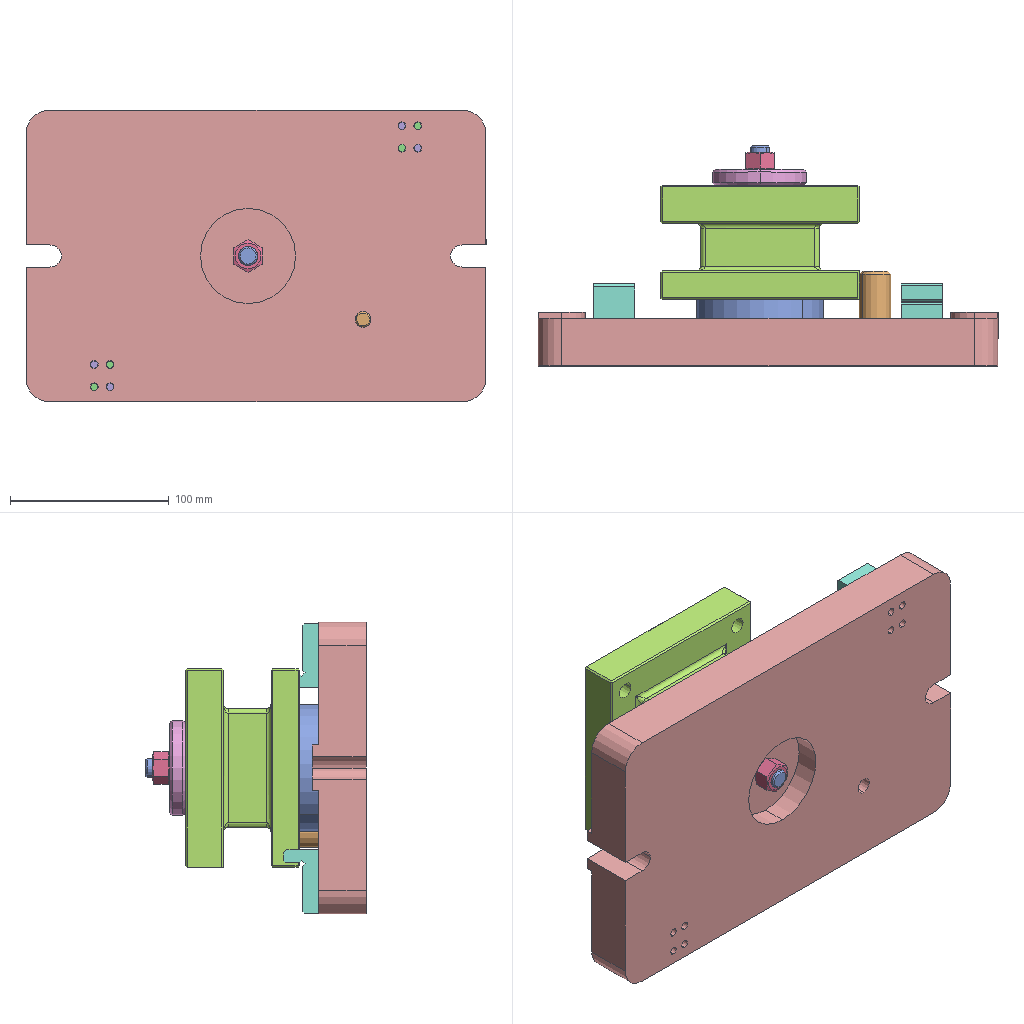Assembly | SolidWorks | 9 different items | 17 placed | box 290 x 139 x 184 mm
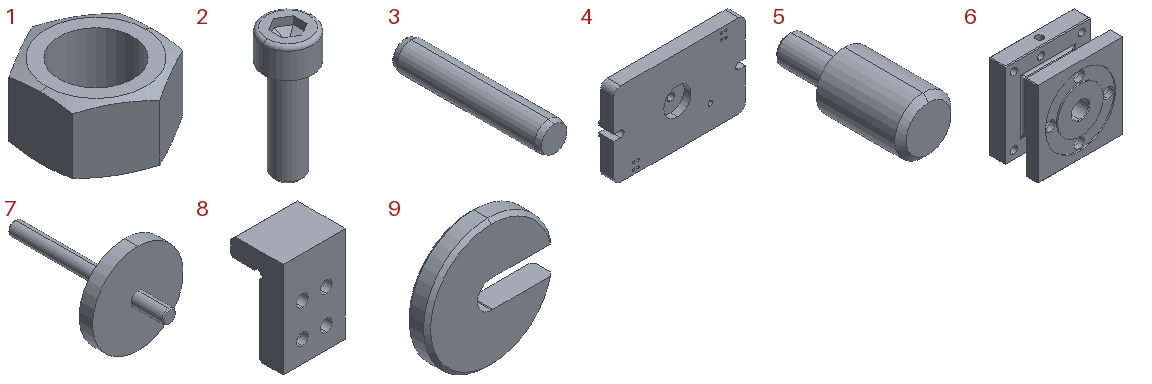Parts list (item | quantity | size | volume | features):
1 | x2 | 18 x 20.785 x 10.8 mm | 1768 mm3 | features Extrusion 1, ICE 1, MirrorPattern 1, RefAxis 1, RevCut 1
2 | x4 | 10 x 10 x 26 mm | 983.883 mm3 | features Chamfer 2, Fillet 2, ICE 2, Extrusion 1, RefAxis 1
3 | x4 | 5 x 26 x 5 mm | 506.42 mm3 | features Chamfer 2, Extrusion 1
4 | x1 | 290 x 34 x 184 mm | 1528919 mm3 | features ICE 7, Fillet 2, Extrusion 1, HoleWzd 1
5 | x1 | 20 x 50 x 20 mm | 10864 mm3 | features Chamfer 2, Extrusion 1, ICE 1
6 | x1 | 125 x 72 x 125 mm | 738027 mm3 | features ICE 7, Fillet 2, HoleWzd 2, Chamfer 1, CirPattern 1, Extrusion 1, RevCut 1
7 | x1 | 80 x 137 x 80 mm | 79942 mm3 | features ICE 2, StudWizard 2, Chamfer 1, Extrusion 1
8 | x2 | 26 x 22 x 40 mm | 10641 mm3 | features Chamfer 2, Cut 2, ICE 2, Extrusion 1, HoleWzd 1
9 | x1 | 59.287 x 10 x 60 mm | 23262 mm3 | features ICE 2, Chamfer 1, Extrusion 1
Mates (type | each side: item.copy, entity, surface, feature):
Concentric | 4.1 face cylinder Cut-Extrude1 | 7.1 face cylinder Boss-Extrude1
Coincident | 4.1 face plane Cut-Extrude3 | 7.1 face plane Boss-Extrude1
Coincident | 7.1 face plane Boss-Extrude1 | 6.1 face plane Boss-Extrude1
Concentric | 7.1 face cylinder Boss-Extrude2 | 6.1 face cylinder Cut-Extrude1
Concentric | 7.1 face cylinder M12 Machine Thread Stud1 | 9.1 face cylinder Boss-Extrude1
Coincident | 6.1 face plane Boss-Extrude3 | 9.1 face plane Boss-Extrude1
Parallel | 4.1 face plane Boss-Extrude1 | 6.1 face plane Boss-Extrude3
Coincident | 4.1 face plane Cut-Extrude3 | 8.1 face plane Boss-Extrude1
DistanceDim | 8.1 face plane Boss-Extrude1 | 4.1 face plane Boss-Extrude1 | 2 times
Concentric | 4.1 face cylinder M6 Tapped Hole1 | 8.2 face cylinder M6 Tapped Hole1
Coincident | 4.1 face plane Cut-Extrude3 | 8.2 face plane Boss-Extrude1
Concentric | 4.1 face cylinder Cut-Extrude5 | 8.2 face cylinder Cut-Extrude2
Concentric | 4.1 face cylinder Cut-Extrude6 | 5.1 face cylinder Boss-Extrude2
Coincident | 4.1 face plane Cut-Extrude3 | 5.1 face plane Boss-Extrude1
Concentric | 8.1 face cylinder Cut-Extrude2 | 3.1 face cylinder Boss-Extrude1
Concentric | 8.1 face cylinder Cut-Extrude2 | 3.2 face cylinder Boss-Extrude1
Coincident | 3.1 face plane Boss-Extrude1 | 3.2 face plane Boss-Extrude1
Coincident | 8.1 face plane Boss-Extrude1 | 3.1 face plane Boss-Extrude1
Concentric | 8.2 face cylinder Cut-Extrude2 | 3.3 face cylinder Boss-Extrude1
Concentric | 8.2 face cylinder Cut-Extrude2 | assembly face
Coincident | 8.2 face plane Boss-Extrude1 | 3.3 face plane Boss-Extrude1
Coincident | 8.2 face plane Boss-Extrude1 | assembly face
Coincident | 8.2 face plane Cut-Extrude3 | 2.1 plane
Concentric | 4.1 face cylinder M6 Tapped Hole1 | 2.1 axis
Coincident | 8.2 face plane Cut-Extrude3 | 2.2 plane
Concentric | 4.1 face cylinder M6 Tapped Hole1 | 2.2 axis
Coincident | 8.2 face plane Cut-Extrude3 | 2.3 plane
Concentric | 4.1 face cylinder M6 Tapped Hole1 | 2.3 axis
Coincident | 8.2 face plane Cut-Extrude3 | 2.4 plane
Concentric | 4.1 face cylinder M6 Tapped Hole1 | 2.4 axis
Coincident | 9.1 face plane Boss-Extrude1 | 1.1 plane
Concentric | 7.1 face cylinder M12 Machine Thread Stud1 | 1.1 axis
Coincident | 4.1 face plane Cut-Extrude2 | 1.2 plane
Concentric | 7.1 face cylinder M12 Machine Thread Stud2 | 1.2 axis
Concentric | 8.2 face cylinder Cut-Extrude2 | 3.4 face cylinder Boss-Extrude1
Coincident | 8.2 face plane Boss-Extrude1 | 3.4 face plane Boss-Extrude1